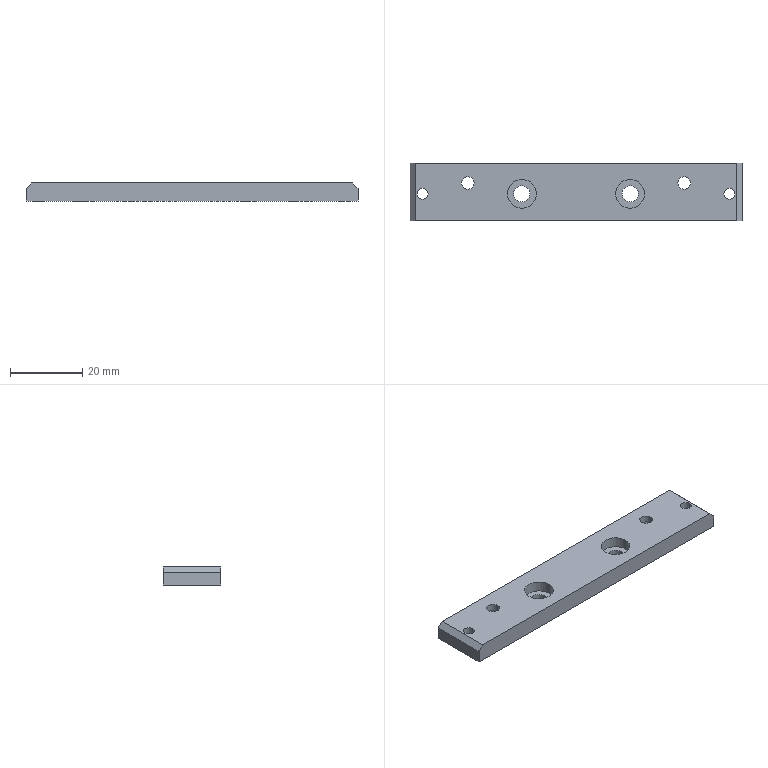Part | NX | 1 solid | 32 faces | box 92 x 16 x 5 mm | volume 6668 mm3 | cylinder 20 | plane 12 | commonest cylinder face diameters 3 x4 3.5 x4 4.5 x4 6.2 x4 8 x4
STEP:
#1=CARTESIAN_POINT('',(-19.,-0.5,-3.));
#2=VERTEX_POINT('',#1);
#3=CARTESIAN_POINT('',(-11.,-0.5,-3.));
#4=VERTEX_POINT('',#3);
#5=CARTESIAN_POINT('',(-15.,-0.5,-3.));
#6=DIRECTION('',(0.,0.,1.));
#7=DIRECTION('',(1.,0.,0.));
#8=AXIS2_PLACEMENT_3D('',#5,#6,#7);
#9=CIRCLE('',#8,4.);
#10=EDGE_CURVE('',#2,#4,#9,.T.);
#11=ORIENTED_EDGE('',*,*,#10,.F.);
#12=CARTESIAN_POINT('',(-19.,-0.5,0.));
#13=VERTEX_POINT('',#12);
#14=CARTESIAN_POINT('',(-19.,-0.5,0.));
#15=DIRECTION('',(0.,0.,1.));
#16=VECTOR('',#15,1000.);
#17=LINE('',#14,#16);
#18=EDGE_CURVE('',#2,#13,#17,.T.);
#19=ORIENTED_EDGE('',*,*,#18,.T.);
#20=CARTESIAN_POINT('',(-11.,-0.5,0.));
#21=VERTEX_POINT('',#20);
#22=CARTESIAN_POINT('',(-15.,-0.5,0.));
#23=DIRECTION('',(0.,0.,1.));
#24=DIRECTION('',(1.,0.,0.));
#25=AXIS2_PLACEMENT_3D('',#22,#23,#24);
#26=CIRCLE('',#25,4.);
#27=EDGE_CURVE('',#13,#21,#26,.T.);
#28=ORIENTED_EDGE('',*,*,#27,.T.);
#29=CARTESIAN_POINT('',(-11.,-0.5,0.));
#30=DIRECTION('',(0.,0.,1.));
#31=VECTOR('',#30,1000.);
#32=LINE('',#29,#31);
#33=EDGE_CURVE('',#4,#21,#32,.T.);
#34=ORIENTED_EDGE('',*,*,#33,.F.);
#35=EDGE_LOOP('',(#11,#19,#28,#34));
#36=FACE_BOUND('',#35,.T.);
#37=CARTESIAN_POINT('',(-15.,-0.5,0.));
#38=DIRECTION('',(0.,0.,1.));
#39=DIRECTION('',(-1.,0.,0.));
#40=AXIS2_PLACEMENT_3D('',#37,#38,#39);
#41=CYLINDRICAL_SURFACE('',#40,4.);
#42=ADVANCED_FACE('',(#36),#41,.F.);
#43=CARTESIAN_POINT('',(-17.25,-0.5,-5.));
#44=VERTEX_POINT('',#43);
#45=CARTESIAN_POINT('',(-12.75,-0.5,-5.));
#46=VERTEX_POINT('',#45);
#47=CARTESIAN_POINT('',(-15.,-0.5,-5.));
#48=DIRECTION('',(0.,0.,1.));
#49=DIRECTION('',(1.,0.,0.));
#50=AXIS2_PLACEMENT_3D('',#47,#48,#49);
#51=CIRCLE('',#50,2.25);
#52=EDGE_CURVE('',#44,#46,#51,.T.);
#53=ORIENTED_EDGE('',*,*,#52,.F.);
#54=CARTESIAN_POINT('',(-17.25,-0.5,-3.));
#55=VERTEX_POINT('',#54);
#56=CARTESIAN_POINT('',(-17.25,-0.5,0.));
#57=DIRECTION('',(0.,0.,1.));
#58=VECTOR('',#57,1000.);
#59=LINE('',#56,#58);
#60=EDGE_CURVE('',#44,#55,#59,.T.);
#61=ORIENTED_EDGE('',*,*,#60,.T.);
#62=CARTESIAN_POINT('',(-12.75,-0.5,-3.));
#63=VERTEX_POINT('',#62);
#64=CARTESIAN_POINT('',(-15.,-0.5,-3.));
#65=DIRECTION('',(0.,0.,1.));
#66=DIRECTION('',(1.,0.,0.));
#67=AXIS2_PLACEMENT_3D('',#64,#65,#66);
#68=CIRCLE('',#67,2.25);
#69=EDGE_CURVE('',#55,#63,#68,.T.);
#70=ORIENTED_EDGE('',*,*,#69,.T.);
#71=CARTESIAN_POINT('',(-12.75,-0.5,0.));
#72=DIRECTION('',(0.,0.,1.));
#73=VECTOR('',#72,1000.);
#74=LINE('',#71,#73);
#75=EDGE_CURVE('',#46,#63,#74,.T.);
#76=ORIENTED_EDGE('',*,*,#75,.F.);
#77=EDGE_LOOP('',(#53,#61,#70,#76));
#78=FACE_BOUND('',#77,.T.);
#79=CARTESIAN_POINT('',(-15.,-0.5,0.));
#80=DIRECTION('',(0.,0.,1.));
#81=DIRECTION('',(-1.,0.,0.));
#82=AXIS2_PLACEMENT_3D('',#79,#80,#81);
#83=CYLINDRICAL_SURFACE('',#82,2.25);
#84=ADVANCED_FACE('',(#78),#83,.F.);
#85=CARTESIAN_POINT('',(11.,-0.5,-3.));
#86=VERTEX_POINT('',#85);
#87=CARTESIAN_POINT('',(19.,-0.5,-3.));
#88=VERTEX_POINT('',#87);
#89=CARTESIAN_POINT('',(15.,-0.5,-3.));
#90=DIRECTION('',(0.,0.,1.));
#91=DIRECTION('',(1.,0.,0.));
#92=AXIS2_PLACEMENT_3D('',#89,#90,#91);
#93=CIRCLE('',#92,4.);
#94=EDGE_CURVE('',#86,#88,#93,.T.);
#95=ORIENTED_EDGE('',*,*,#94,.F.);
#96=CARTESIAN_POINT('',(11.,-0.5,0.));
#97=VERTEX_POINT('',#96);
#98=CARTESIAN_POINT('',(11.,-0.5,0.));
#99=DIRECTION('',(0.,0.,1.));
#100=VECTOR('',#99,1000.);
#101=LINE('',#98,#100);
#102=EDGE_CURVE('',#86,#97,#101,.T.);
#103=ORIENTED_EDGE('',*,*,#102,.T.);
#104=CARTESIAN_POINT('',(19.,-0.5,0.));
#105=VERTEX_POINT('',#104);
#106=CARTESIAN_POINT('',(15.,-0.5,0.));
#107=DIRECTION('',(0.,0.,1.));
#108=DIRECTION('',(1.,0.,0.));
#109=AXIS2_PLACEMENT_3D('',#106,#107,#108);
#110=CIRCLE('',#109,4.);
#111=EDGE_CURVE('',#97,#105,#110,.T.);
#112=ORIENTED_EDGE('',*,*,#111,.T.);
#113=CARTESIAN_POINT('',(19.,-0.5,0.));
#114=DIRECTION('',(0.,0.,1.));
#115=VECTOR('',#114,1000.);
#116=LINE('',#113,#115);
#117=EDGE_CURVE('',#88,#105,#116,.T.);
#118=ORIENTED_EDGE('',*,*,#117,.F.);
#119=EDGE_LOOP('',(#95,#103,#112,#118));
#120=FACE_BOUND('',#119,.T.);
#121=CARTESIAN_POINT('',(15.,-0.5,0.));
#122=DIRECTION('',(0.,0.,1.));
#123=DIRECTION('',(-1.,0.,0.));
#124=AXIS2_PLACEMENT_3D('',#121,#122,#123);
#125=CYLINDRICAL_SURFACE('',#124,4.);
#126=ADVANCED_FACE('',(#120),#125,.F.);
#127=CARTESIAN_POINT('',(12.75,-0.5,-5.));
#128=VERTEX_POINT('',#127);
#129=CARTESIAN_POINT('',(17.25,-0.5,-5.));
#130=VERTEX_POINT('',#129);
#131=CARTESIAN_POINT('',(15.,-0.5,-5.));
#132=DIRECTION('',(0.,0.,1.));
#133=DIRECTION('',(1.,0.,0.));
#134=AXIS2_PLACEMENT_3D('',#131,#132,#133);
#135=CIRCLE('',#134,2.25);
#136=EDGE_CURVE('',#128,#130,#135,.T.);
#137=ORIENTED_EDGE('',*,*,#136,.F.);
#138=CARTESIAN_POINT('',(12.75,-0.5,-3.));
#139=VERTEX_POINT('',#138);
#140=CARTESIAN_POINT('',(12.75,-0.5,0.));
#141=DIRECTION('',(0.,0.,1.));
#142=VECTOR('',#141,1000.);
#143=LINE('',#140,#142);
#144=EDGE_CURVE('',#128,#139,#143,.T.);
#145=ORIENTED_EDGE('',*,*,#144,.T.);
#146=CARTESIAN_POINT('',(17.25,-0.5,-3.));
#147=VERTEX_POINT('',#146);
#148=CARTESIAN_POINT('',(15.,-0.5,-3.));
#149=DIRECTION('',(0.,0.,1.));
#150=DIRECTION('',(1.,0.,0.));
#151=AXIS2_PLACEMENT_3D('',#148,#149,#150);
#152=CIRCLE('',#151,2.25);
#153=EDGE_CURVE('',#139,#147,#152,.T.);
#154=ORIENTED_EDGE('',*,*,#153,.T.);
#155=CARTESIAN_POINT('',(17.25,-0.5,0.));
#156=DIRECTION('',(0.,0.,1.));
#157=VECTOR('',#156,1000.);
#158=LINE('',#155,#157);
#159=EDGE_CURVE('',#130,#147,#158,.T.);
#160=ORIENTED_EDGE('',*,*,#159,.F.);
#161=EDGE_LOOP('',(#137,#145,#154,#160));
#162=FACE_BOUND('',#161,.T.);
#163=CARTESIAN_POINT('',(15.,-0.5,0.));
#164=DIRECTION('',(0.,0.,1.));
#165=DIRECTION('',(-1.,0.,0.));
#166=AXIS2_PLACEMENT_3D('',#163,#164,#165);
#167=CYLINDRICAL_SURFACE('',#166,2.25);
#168=ADVANCED_FACE('',(#162),#167,.F.);
#169=CARTESIAN_POINT('',(-41.,-0.5,0.));
#170=VERTEX_POINT('',#169);
#171=CARTESIAN_POINT('',(-44.,-0.5,0.));
#172=VERTEX_POINT('',#171);
#173=CARTESIAN_POINT('',(-42.5,-0.5,0.));
#174=DIRECTION('',(0.,0.,-1.));
#175=DIRECTION('',(-1.,0.,0.));
#176=AXIS2_PLACEMENT_3D('',#173,#174,#175);
#177=CIRCLE('',#176,1.5);
#178=EDGE_CURVE('',#170,#172,#177,.T.);
#179=ORIENTED_EDGE('',*,*,#178,.F.);
#180=CARTESIAN_POINT('',(-41.,-0.5,-5.));
#181=VERTEX_POINT('',#180);
#182=CARTESIAN_POINT('',(-41.,-0.5,-5.));
#183=DIRECTION('',(0.,0.,-1.));
#184=VECTOR('',#183,1000.);
#185=LINE('',#182,#184);
#186=EDGE_CURVE('',#170,#181,#185,.T.);
#187=ORIENTED_EDGE('',*,*,#186,.T.);
#188=CARTESIAN_POINT('',(-44.,-0.5,-5.));
#189=VERTEX_POINT('',#188);
#190=CARTESIAN_POINT('',(-42.5,-0.5,-5.));
#191=DIRECTION('',(0.,0.,-1.));
#192=DIRECTION('',(-1.,0.,0.));
#193=AXIS2_PLACEMENT_3D('',#190,#191,#192);
#194=CIRCLE('',#193,1.5);
#195=EDGE_CURVE('',#181,#189,#194,.T.);
#196=ORIENTED_EDGE('',*,*,#195,.T.);
#197=CARTESIAN_POINT('',(-44.,-0.5,-5.));
#198=DIRECTION('',(0.,0.,-1.));
#199=VECTOR('',#198,1000.);
#200=LINE('',#197,#199);
#201=EDGE_CURVE('',#172,#189,#200,.T.);
#202=ORIENTED_EDGE('',*,*,#201,.F.);
#203=EDGE_LOOP('',(#179,#187,#196,#202));
#204=FACE_BOUND('',#203,.T.);
#205=CARTESIAN_POINT('',(-42.5,-0.5,-5.));
#206=DIRECTION('',(0.,0.,-1.));
#207=DIRECTION('',(1.,0.,0.));
#208=AXIS2_PLACEMENT_3D('',#205,#206,#207);
#209=CYLINDRICAL_SURFACE('',#208,1.5);
#210=ADVANCED_FACE('',(#204),#209,.F.);
#211=CARTESIAN_POINT('',(44.,-0.5,0.));
#212=VERTEX_POINT('',#211);
#213=CARTESIAN_POINT('',(41.,-0.5,0.));
#214=VERTEX_POINT('',#213);
#215=CARTESIAN_POINT('',(42.5,-0.5,0.));
#216=DIRECTION('',(0.,0.,-1.));
#217=DIRECTION('',(-1.,0.,0.));
#218=AXIS2_PLACEMENT_3D('',#215,#216,#217);
#219=CIRCLE('',#218,1.5);
#220=EDGE_CURVE('',#212,#214,#219,.T.);
#221=ORIENTED_EDGE('',*,*,#220,.F.);
#222=CARTESIAN_POINT('',(44.,-0.5,-5.));
#223=VERTEX_POINT('',#222);
#224=CARTESIAN_POINT('',(44.,-0.5,-5.));
#225=DIRECTION('',(0.,0.,-1.));
#226=VECTOR('',#225,1000.);
#227=LINE('',#224,#226);
#228=EDGE_CURVE('',#212,#223,#227,.T.);
#229=ORIENTED_EDGE('',*,*,#228,.T.);
#230=CARTESIAN_POINT('',(41.,-0.5,-5.));
#231=VERTEX_POINT('',#230);
#232=CARTESIAN_POINT('',(42.5,-0.5,-5.));
#233=DIRECTION('',(0.,0.,-1.));
#234=DIRECTION('',(-1.,0.,0.));
#235=AXIS2_PLACEMENT_3D('',#232,#233,#234);
#236=CIRCLE('',#235,1.5);
#237=EDGE_CURVE('',#223,#231,#236,.T.);
#238=ORIENTED_EDGE('',*,*,#237,.T.);
#239=CARTESIAN_POINT('',(41.,-0.5,-5.));
#240=DIRECTION('',(0.,0.,-1.));
#241=VECTOR('',#240,1000.);
#242=LINE('',#239,#241);
#243=EDGE_CURVE('',#214,#231,#242,.T.);
#244=ORIENTED_EDGE('',*,*,#243,.F.);
#245=EDGE_LOOP('',(#221,#229,#238,#244));
#246=FACE_BOUND('',#245,.T.);
#247=CARTESIAN_POINT('',(42.5,-0.5,-5.));
#248=DIRECTION('',(0.,0.,-1.));
#249=DIRECTION('',(1.,0.,0.));
#250=AXIS2_PLACEMENT_3D('',#247,#248,#249);
#251=CYLINDRICAL_SURFACE('',#250,1.5);
#252=ADVANCED_FACE('',(#246),#251,.F.);
#253=CARTESIAN_POINT('',(-31.75,2.5,0.));
#254=VERTEX_POINT('',#253);
#255=CARTESIAN_POINT('',(-28.25,2.5,0.));
#256=VERTEX_POINT('',#255);
#257=CARTESIAN_POINT('',(-30.,2.5,0.));
#258=DIRECTION('',(0.,0.,1.));
#259=DIRECTION('',(1.,0.,0.));
#260=AXIS2_PLACEMENT_3D('',#257,#258,#259);
#261=CIRCLE('',#260,1.75);
#262=EDGE_CURVE('',#254,#256,#261,.T.);
#263=ORIENTED_EDGE('',*,*,#262,.T.);
#264=CARTESIAN_POINT('',(-28.25,2.5,-2.));
#265=VERTEX_POINT('',#264);
#266=CARTESIAN_POINT('',(-28.25,2.5,-2.));
#267=DIRECTION('',(0.,0.,-1.));
#268=VECTOR('',#267,1000.);
#269=LINE('',#266,#268);
#270=EDGE_CURVE('',#256,#265,#269,.T.);
#271=ORIENTED_EDGE('',*,*,#270,.T.);
#272=CARTESIAN_POINT('',(-31.75,2.5,-2.));
#273=VERTEX_POINT('',#272);
#274=CARTESIAN_POINT('',(-30.,2.5,-2.));
#275=DIRECTION('',(0.,0.,-1.));
#276=DIRECTION('',(-1.,0.,0.));
#277=AXIS2_PLACEMENT_3D('',#274,#275,#276);
#278=CIRCLE('',#277,1.75);
#279=EDGE_CURVE('',#265,#273,#278,.T.);
#280=ORIENTED_EDGE('',*,*,#279,.T.);
#281=CARTESIAN_POINT('',(-31.75,2.5,-2.));
#282=DIRECTION('',(0.,0.,-1.));
#283=VECTOR('',#282,1000.);
#284=LINE('',#281,#283);
#285=EDGE_CURVE('',#254,#273,#284,.T.);
#286=ORIENTED_EDGE('',*,*,#285,.F.);
#287=EDGE_LOOP('',(#263,#271,#280,#286));
#288=FACE_BOUND('',#287,.T.);
#289=CARTESIAN_POINT('',(-30.,2.5,-2.));
#290=DIRECTION('',(0.,0.,-1.));
#291=DIRECTION('',(1.,0.,0.));
#292=AXIS2_PLACEMENT_3D('',#289,#290,#291);
#293=CYLINDRICAL_SURFACE('',#292,1.75);
#294=ADVANCED_FACE('',(#288),#293,.F.);
#295=CARTESIAN_POINT('',(28.25,2.5,0.));
#296=VERTEX_POINT('',#295);
#297=CARTESIAN_POINT('',(31.75,2.5,0.));
#298=VERTEX_POINT('',#297);
#299=CARTESIAN_POINT('',(30.,2.5,0.));
#300=DIRECTION('',(0.,0.,1.));
#301=DIRECTION('',(1.,0.,0.));
#302=AXIS2_PLACEMENT_3D('',#299,#300,#301);
#303=CIRCLE('',#302,1.75);
#304=EDGE_CURVE('',#296,#298,#303,.T.);
#305=ORIENTED_EDGE('',*,*,#304,.T.);
#306=CARTESIAN_POINT('',(31.75,2.5,-2.));
#307=VERTEX_POINT('',#306);
#308=CARTESIAN_POINT('',(31.75,2.5,-2.));
#309=DIRECTION('',(0.,0.,-1.));
#310=VECTOR('',#309,1000.);
#311=LINE('',#308,#310);
#312=EDGE_CURVE('',#298,#307,#311,.T.);
#313=ORIENTED_EDGE('',*,*,#312,.T.);
#314=CARTESIAN_POINT('',(28.25,2.5,-2.));
#315=VERTEX_POINT('',#314);
#316=CARTESIAN_POINT('',(30.,2.5,-2.));
#317=DIRECTION('',(0.,0.,-1.));
#318=DIRECTION('',(-1.,0.,0.));
#319=AXIS2_PLACEMENT_3D('',#316,#317,#318);
#320=CIRCLE('',#319,1.75);
#321=EDGE_CURVE('',#307,#315,#320,.T.);
#322=ORIENTED_EDGE('',*,*,#321,.T.);
#323=CARTESIAN_POINT('',(28.25,2.5,-2.));
#324=DIRECTION('',(0.,0.,-1.));
#325=VECTOR('',#324,1000.);
#326=LINE('',#323,#325);
#327=EDGE_CURVE('',#296,#315,#326,.T.);
#328=ORIENTED_EDGE('',*,*,#327,.F.);
#329=EDGE_LOOP('',(#305,#313,#322,#328));
#330=FACE_BOUND('',#329,.T.);
#331=CARTESIAN_POINT('',(30.,2.5,-2.));
#332=DIRECTION('',(0.,0.,-1.));
#333=DIRECTION('',(1.,0.,0.));
#334=AXIS2_PLACEMENT_3D('',#331,#332,#333);
#335=CYLINDRICAL_SURFACE('',#334,1.75);
#336=ADVANCED_FACE('',(#330),#335,.F.);
#337=CARTESIAN_POINT('',(26.9,2.5,-2.));
#338=VERTEX_POINT('',#337);
#339=CARTESIAN_POINT('',(33.1,2.5,-2.));
#340=VERTEX_POINT('',#339);
#341=CARTESIAN_POINT('',(30.,2.5,-2.));
#342=DIRECTION('',(0.,0.,1.));
#343=DIRECTION('',(1.,0.,0.));
#344=AXIS2_PLACEMENT_3D('',#341,#342,#343);
#345=CIRCLE('',#344,3.1);
#346=EDGE_CURVE('',#338,#340,#345,.T.);
#347=ORIENTED_EDGE('',*,*,#346,.T.);
#348=CARTESIAN_POINT('',(33.1,2.5,-5.));
#349=VERTEX_POINT('',#348);
#350=CARTESIAN_POINT('',(33.1,2.5,-2.));
#351=DIRECTION('',(0.,0.,-1.));
#352=VECTOR('',#351,1000.);
#353=LINE('',#350,#352);
#354=EDGE_CURVE('',#340,#349,#353,.T.);
#355=ORIENTED_EDGE('',*,*,#354,.T.);
#356=CARTESIAN_POINT('',(26.9,2.5,-5.));
#357=VERTEX_POINT('',#356);
#358=CARTESIAN_POINT('',(30.,2.5,-5.));
#359=DIRECTION('',(0.,0.,1.));
#360=DIRECTION('',(1.,0.,0.));
#361=AXIS2_PLACEMENT_3D('',#358,#359,#360);
#362=CIRCLE('',#361,3.1);
#363=EDGE_CURVE('',#357,#349,#362,.T.);
#364=ORIENTED_EDGE('',*,*,#363,.F.);
#365=CARTESIAN_POINT('',(26.9,2.5,-2.));
#366=DIRECTION('',(0.,0.,-1.));
#367=VECTOR('',#366,1000.);
#368=LINE('',#365,#367);
#369=EDGE_CURVE('',#338,#357,#368,.T.);
#370=ORIENTED_EDGE('',*,*,#369,.F.);
#371=EDGE_LOOP('',(#347,#355,#364,#370));
#372=FACE_BOUND('',#371,.T.);
#373=CARTESIAN_POINT('',(30.,2.5,-2.));
#374=DIRECTION('',(0.,0.,-1.));
#375=DIRECTION('',(1.,0.,0.));
#376=AXIS2_PLACEMENT_3D('',#373,#374,#375);
#377=CYLINDRICAL_SURFACE('',#376,3.1);
#378=ADVANCED_FACE('',(#372),#377,.F.);
#379=CARTESIAN_POINT('',(-33.1,2.5,-2.));
#380=VERTEX_POINT('',#379);
#381=CARTESIAN_POINT('',(-26.9,2.5,-2.));
#382=VERTEX_POINT('',#381);
#383=CARTESIAN_POINT('',(-30.,2.5,-2.));
#384=DIRECTION('',(0.,0.,1.));
#385=DIRECTION('',(1.,0.,0.));
#386=AXIS2_PLACEMENT_3D('',#383,#384,#385);
#387=CIRCLE('',#386,3.1);
#388=EDGE_CURVE('',#380,#382,#387,.T.);
#389=ORIENTED_EDGE('',*,*,#388,.T.);
#390=CARTESIAN_POINT('',(-26.9,2.5,-5.));
#391=VERTEX_POINT('',#390);
#392=CARTESIAN_POINT('',(-26.9,2.5,-2.));
#393=DIRECTION('',(0.,0.,-1.));
#394=VECTOR('',#393,1000.);
#395=LINE('',#392,#394);
#396=EDGE_CURVE('',#382,#391,#395,.T.);
#397=ORIENTED_EDGE('',*,*,#396,.T.);
#398=CARTESIAN_POINT('',(-33.1,2.5,-5.));
#399=VERTEX_POINT('',#398);
#400=CARTESIAN_POINT('',(-30.,2.5,-5.));
#401=DIRECTION('',(0.,0.,1.));
#402=DIRECTION('',(1.,0.,0.));
#403=AXIS2_PLACEMENT_3D('',#400,#401,#402);
#404=CIRCLE('',#403,3.1);
#405=EDGE_CURVE('',#399,#391,#404,.T.);
#406=ORIENTED_EDGE('',*,*,#405,.F.);
#407=CARTESIAN_POINT('',(-33.1,2.5,-2.));
#408=DIRECTION('',(0.,0.,-1.));
#409=VECTOR('',#408,1000.);
#410=LINE('',#407,#409);
#411=EDGE_CURVE('',#380,#399,#410,.T.);
#412=ORIENTED_EDGE('',*,*,#411,.F.);
#413=EDGE_LOOP('',(#389,#397,#406,#412));
#414=FACE_BOUND('',#413,.T.);
#415=CARTESIAN_POINT('',(-30.,2.5,-2.));
#416=DIRECTION('',(0.,0.,-1.));
#417=DIRECTION('',(1.,0.,0.));
#418=AXIS2_PLACEMENT_3D('',#415,#416,#417);
#419=CYLINDRICAL_SURFACE('',#418,3.1);
#420=ADVANCED_FACE('',(#414),#419,.F.);
#421=ORIENTED_EDGE('',*,*,#388,.F.);
#422=CARTESIAN_POINT('',(-30.,2.5,-2.));
#423=DIRECTION('',(0.,0.,1.));
#424=DIRECTION('',(1.,0.,0.));
#425=AXIS2_PLACEMENT_3D('',#422,#423,#424);
#426=CIRCLE('',#425,3.1);
#427=EDGE_CURVE('',#382,#380,#426,.T.);
#428=ORIENTED_EDGE('',*,*,#427,.F.);
#429=EDGE_LOOP('',(#421,#428));
#430=FACE_BOUND('',#429,.T.);
#431=CARTESIAN_POINT('',(-30.,2.5,-2.));
#432=DIRECTION('',(0.,0.,-1.));
#433=DIRECTION('',(-1.,0.,0.));
#434=AXIS2_PLACEMENT_3D('',#431,#432,#433);
#435=CIRCLE('',#434,1.75);
#436=EDGE_CURVE('',#273,#265,#435,.T.);
#437=ORIENTED_EDGE('',*,*,#436,.F.);
#438=ORIENTED_EDGE('',*,*,#279,.F.);
#439=EDGE_LOOP('',(#437,#438));
#440=FACE_BOUND('',#439,.T.);
#441=CARTESIAN_POINT('',(-30.,2.5,-2.));
#442=DIRECTION('',(0.,0.,1.));
#443=DIRECTION('',(-1.,0.,0.));
#444=AXIS2_PLACEMENT_3D('',#441,#442,#443);
#445=PLANE('',#444);
#446=ADVANCED_FACE('',(#430,#440),#445,.F.);
#447=CARTESIAN_POINT('',(46.,8.,-1.5));
#448=VERTEX_POINT('',#447);
#449=CARTESIAN_POINT('',(46.,8.,-5.));
#450=VERTEX_POINT('',#449);
#451=CARTESIAN_POINT('',(46.,8.,0.));
#452=DIRECTION('',(0.,0.,-1.));
#453=VECTOR('',#452,1000.);
#454=LINE('',#451,#453);
#455=EDGE_CURVE('',#448,#450,#454,.T.);
#456=ORIENTED_EDGE('',*,*,#455,.F.);
#457=CARTESIAN_POINT('',(46.,-8.,-1.5));
#458=VERTEX_POINT('',#457);
#459=CARTESIAN_POINT('',(46.,-8.,-1.5));
#460=DIRECTION('',(0.,-1.,0.));
#461=VECTOR('',#460,1000.);
#462=LINE('',#459,#461);
#463=EDGE_CURVE('',#448,#458,#462,.T.);
#464=ORIENTED_EDGE('',*,*,#463,.T.);
#465=CARTESIAN_POINT('',(46.,-8.,-5.));
#466=VERTEX_POINT('',#465);
#467=CARTESIAN_POINT('',(46.,-8.,0.));
#468=DIRECTION('',(0.,0.,-1.));
#469=VECTOR('',#468,1000.);
#470=LINE('',#467,#469);
#471=EDGE_CURVE('',#458,#466,#470,.T.);
#472=ORIENTED_EDGE('',*,*,#471,.T.);
#473=CARTESIAN_POINT('',(46.,8.,-5.));
#474=DIRECTION('',(0.,1.,0.));
#475=VECTOR('',#474,1000.);
#476=LINE('',#473,#475);
#477=EDGE_CURVE('',#466,#450,#476,.T.);
#478=ORIENTED_EDGE('',*,*,#477,.T.);
#479=EDGE_LOOP('',(#456,#464,#472,#478));
#480=FACE_BOUND('',#479,.T.);
#481=CARTESIAN_POINT('',(46.,8.,0.));
#482=DIRECTION('',(-1.,0.,0.));
#483=DIRECTION('',(0.,0.,-1.));
#484=AXIS2_PLACEMENT_3D('',#481,#482,#483);
#485=PLANE('',#484);
#486=ADVANCED_FACE('',(#480),#485,.F.);
#487=CARTESIAN_POINT('',(-46.,8.,-1.5));
#488=VERTEX_POINT('',#487);
#489=CARTESIAN_POINT('',(-46.,8.,-5.));
#490=VERTEX_POINT('',#489);
#491=CARTESIAN_POINT('',(-46.,8.,0.));
#492=DIRECTION('',(0.,0.,-1.));
#493=VECTOR('',#492,1000.);
#494=LINE('',#491,#493);
#495=EDGE_CURVE('',#488,#490,#494,.T.);
#496=ORIENTED_EDGE('',*,*,#495,.F.);
#497=CARTESIAN_POINT('',(-44.5,8.,0.));
#498=VERTEX_POINT('',#497);
#499=CARTESIAN_POINT('',(-44.5,8.,0.));
#500=DIRECTION('',(0.7071,0.,0.7071));
#501=VECTOR('',#500,1000.);
#502=LINE('',#499,#501);
#503=EDGE_CURVE('',#488,#498,#502,.T.);
#504=ORIENTED_EDGE('',*,*,#503,.T.);
#505=CARTESIAN_POINT('',(44.5,8.,0.));
#506=VERTEX_POINT('',#505);
#507=CARTESIAN_POINT('',(-46.,8.,0.));
#508=DIRECTION('',(-1.,0.,0.));
#509=VECTOR('',#508,1000.);
#510=LINE('',#507,#509);
#511=EDGE_CURVE('',#506,#498,#510,.T.);
#512=ORIENTED_EDGE('',*,*,#511,.F.);
#513=CARTESIAN_POINT('',(44.5,8.,0.));
#514=DIRECTION('',(0.7071,0.,-0.7071));
#515=VECTOR('',#514,1000.);
#516=LINE('',#513,#515);
#517=EDGE_CURVE('',#506,#448,#516,.T.);
#518=ORIENTED_EDGE('',*,*,#517,.T.);
#519=ORIENTED_EDGE('',*,*,#455,.T.);
#520=CARTESIAN_POINT('',(-46.,8.,-5.));
#521=DIRECTION('',(-1.,0.,0.));
#522=VECTOR('',#521,1000.);
#523=LINE('',#520,#522);
#524=EDGE_CURVE('',#450,#490,#523,.T.);
#525=ORIENTED_EDGE('',*,*,#524,.T.);
#526=EDGE_LOOP('',(#496,#504,#512,#518,#519,#525));
#527=FACE_BOUND('',#526,.T.);
#528=CARTESIAN_POINT('',(-46.,8.,0.));
#529=DIRECTION('',(0.,-1.,0.));
#530=DIRECTION('',(0.,0.,1.));
#531=AXIS2_PLACEMENT_3D('',#528,#529,#530);
#532=PLANE('',#531);
#533=ADVANCED_FACE('',(#527),#532,.F.);
#534=CARTESIAN_POINT('',(-46.,-8.,-1.5));
#535=VERTEX_POINT('',#534);
#536=CARTESIAN_POINT('',(-46.,-8.,-5.));
#537=VERTEX_POINT('',#536);
#538=CARTESIAN_POINT('',(-46.,-8.,0.));
#539=DIRECTION('',(0.,0.,-1.));
#540=VECTOR('',#539,1000.);
#541=LINE('',#538,#540);
#542=EDGE_CURVE('',#535,#537,#541,.T.);
#543=ORIENTED_EDGE('',*,*,#542,.F.);
#544=CARTESIAN_POINT('',(-46.,8.,-1.5));
#545=DIRECTION('',(0.,1.,0.));
#546=VECTOR('',#545,1000.);
#547=LINE('',#544,#546);
#548=EDGE_CURVE('',#535,#488,#547,.T.);
#549=ORIENTED_EDGE('',*,*,#548,.T.);
#550=ORIENTED_EDGE('',*,*,#495,.T.);
#551=CARTESIAN_POINT('',(-46.,8.,-5.));
#552=DIRECTION('',(0.,-1.,0.));
#553=VECTOR('',#552,1000.);
#554=LINE('',#551,#553);
#555=EDGE_CURVE('',#490,#537,#554,.T.);
#556=ORIENTED_EDGE('',*,*,#555,.T.);
#557=EDGE_LOOP('',(#543,#549,#550,#556));
#558=FACE_BOUND('',#557,.T.);
#559=CARTESIAN_POINT('',(-46.,8.,0.));
#560=DIRECTION('',(1.,0.,0.));
#561=DIRECTION('',(0.,0.,1.));
#562=AXIS2_PLACEMENT_3D('',#559,#560,#561);
#563=PLANE('',#562);
#564=ADVANCED_FACE('',(#558),#563,.F.);
#565=CARTESIAN_POINT('',(-44.5,-8.,0.));
#566=VERTEX_POINT('',#565);
#567=CARTESIAN_POINT('',(44.5,-8.,0.));
#568=VERTEX_POINT('',#567);
#569=CARTESIAN_POINT('',(-46.,-8.,0.));
#570=DIRECTION('',(1.,0.,0.));
#571=VECTOR('',#570,1000.);
#572=LINE('',#569,#571);
#573=EDGE_CURVE('',#566,#568,#572,.T.);
#574=ORIENTED_EDGE('',*,*,#573,.F.);
#575=CARTESIAN_POINT('',(-44.5,-8.,0.));
#576=DIRECTION('',(-0.7071,0.,-0.7071));
#577=VECTOR('',#576,1000.);
#578=LINE('',#575,#577);
#579=EDGE_CURVE('',#566,#535,#578,.T.);
#580=ORIENTED_EDGE('',*,*,#579,.T.);
#581=ORIENTED_EDGE('',*,*,#542,.T.);
#582=CARTESIAN_POINT('',(-46.,-8.,-5.));
#583=DIRECTION('',(1.,0.,0.));
#584=VECTOR('',#583,1000.);
#585=LINE('',#582,#584);
#586=EDGE_CURVE('',#537,#466,#585,.T.);
#587=ORIENTED_EDGE('',*,*,#586,.T.);
#588=ORIENTED_EDGE('',*,*,#471,.F.);
#589=CARTESIAN_POINT('',(44.5,-8.,0.));
#590=DIRECTION('',(-0.7071,0.,0.7071));
#591=VECTOR('',#590,1000.);
#592=LINE('',#589,#591);
#593=EDGE_CURVE('',#458,#568,#592,.T.);
#594=ORIENTED_EDGE('',*,*,#593,.T.);
#595=EDGE_LOOP('',(#574,#580,#581,#587,#588,#594));
#596=FACE_BOUND('',#595,.T.);
#597=CARTESIAN_POINT('',(-46.,-8.,0.));
#598=DIRECTION('',(0.,1.,0.));
#599=DIRECTION('',(0.,0.,-1.));
#600=AXIS2_PLACEMENT_3D('',#597,#598,#599);
#601=PLANE('',#600);
#602=ADVANCED_FACE('',(#596),#601,.F.);
#603=CARTESIAN_POINT('',(-15.,-0.5,0.));
#604=DIRECTION('',(0.,0.,1.));
#605=DIRECTION('',(1.,0.,0.));
#606=AXIS2_PLACEMENT_3D('',#603,#604,#605);
#607=CIRCLE('',#606,4.);
#608=EDGE_CURVE('',#21,#13,#607,.T.);
#609=ORIENTED_EDGE('',*,*,#608,.F.);
#610=ORIENTED_EDGE('',*,*,#27,.F.);
#611=EDGE_LOOP('',(#609,#610));
#612=FACE_BOUND('',#611,.T.);
#613=CARTESIAN_POINT('',(15.,-0.5,0.));
#614=DIRECTION('',(0.,0.,1.));
#615=DIRECTION('',(1.,0.,0.));
#616=AXIS2_PLACEMENT_3D('',#613,#614,#615);
#617=CIRCLE('',#616,4.);
#618=EDGE_CURVE('',#105,#97,#617,.T.);
#619=ORIENTED_EDGE('',*,*,#618,.F.);
#620=ORIENTED_EDGE('',*,*,#111,.F.);
#621=EDGE_LOOP('',(#619,#620));
#622=FACE_BOUND('',#621,.T.);
#623=CARTESIAN_POINT('',(-42.5,-0.5,0.));
#624=DIRECTION('',(0.,0.,-1.));
#625=DIRECTION('',(-1.,0.,0.));
#626=AXIS2_PLACEMENT_3D('',#623,#624,#625);
#627=CIRCLE('',#626,1.5);
#628=EDGE_CURVE('',#172,#170,#627,.T.);
#629=ORIENTED_EDGE('',*,*,#628,.T.);
#630=ORIENTED_EDGE('',*,*,#178,.T.);
#631=EDGE_LOOP('',(#629,#630));
#632=FACE_BOUND('',#631,.T.);
#633=CARTESIAN_POINT('',(42.5,-0.5,0.));
#634=DIRECTION('',(0.,0.,-1.));
#635=DIRECTION('',(-1.,0.,0.));
#636=AXIS2_PLACEMENT_3D('',#633,#634,#635);
#637=CIRCLE('',#636,1.5);
#638=EDGE_CURVE('',#214,#212,#637,.T.);
#639=ORIENTED_EDGE('',*,*,#638,.T.);
#640=ORIENTED_EDGE('',*,*,#220,.T.);
#641=EDGE_LOOP('',(#639,#640));
#642=FACE_BOUND('',#641,.T.);
#643=ORIENTED_EDGE('',*,*,#262,.F.);
#644=CARTESIAN_POINT('',(-30.,2.5,0.));
#645=DIRECTION('',(0.,0.,1.));
#646=DIRECTION('',(1.,0.,0.));
#647=AXIS2_PLACEMENT_3D('',#644,#645,#646);
#648=CIRCLE('',#647,1.75);
#649=EDGE_CURVE('',#256,#254,#648,.T.);
#650=ORIENTED_EDGE('',*,*,#649,.F.);
#651=EDGE_LOOP('',(#643,#650));
#652=FACE_BOUND('',#651,.T.);
#653=ORIENTED_EDGE('',*,*,#304,.F.);
#654=CARTESIAN_POINT('',(30.,2.5,0.));
#655=DIRECTION('',(0.,0.,1.));
#656=DIRECTION('',(1.,0.,0.));
#657=AXIS2_PLACEMENT_3D('',#654,#655,#656);
#658=CIRCLE('',#657,1.75);
#659=EDGE_CURVE('',#298,#296,#658,.T.);
#660=ORIENTED_EDGE('',*,*,#659,.F.);
#661=EDGE_LOOP('',(#653,#660));
#662=FACE_BOUND('',#661,.T.);
#663=ORIENTED_EDGE('',*,*,#511,.T.);
#664=CARTESIAN_POINT('',(-44.5,-8.,0.));
#665=DIRECTION('',(0.,-1.,0.));
#666=VECTOR('',#665,1000.);
#667=LINE('',#664,#666);
#668=EDGE_CURVE('',#498,#566,#667,.T.);
#669=ORIENTED_EDGE('',*,*,#668,.T.);
#670=ORIENTED_EDGE('',*,*,#573,.T.);
#671=CARTESIAN_POINT('',(44.5,8.,0.));
#672=DIRECTION('',(0.,1.,0.));
#673=VECTOR('',#672,1000.);
#674=LINE('',#671,#673);
#675=EDGE_CURVE('',#568,#506,#674,.T.);
#676=ORIENTED_EDGE('',*,*,#675,.T.);
#677=EDGE_LOOP('',(#663,#669,#670,#676));
#678=FACE_BOUND('',#677,.T.);
#679=CARTESIAN_POINT('',(0.,0.,0.));
#680=DIRECTION('',(0.,0.,1.));
#681=DIRECTION('',(-1.,0.,0.));
#682=AXIS2_PLACEMENT_3D('',#679,#680,#681);
#683=PLANE('',#682);
#684=ADVANCED_FACE('',(#612,#622,#632,#642,#652,#662,#678),#683,.T.);
#685=CARTESIAN_POINT('',(-15.,-0.5,-5.));
#686=DIRECTION('',(0.,0.,1.));
#687=DIRECTION('',(1.,0.,0.));
#688=AXIS2_PLACEMENT_3D('',#685,#686,#687);
#689=CIRCLE('',#688,2.25);
#690=EDGE_CURVE('',#46,#44,#689,.T.);
#691=ORIENTED_EDGE('',*,*,#690,.T.);
#692=ORIENTED_EDGE('',*,*,#52,.T.);
#693=EDGE_LOOP('',(#691,#692));
#694=FACE_BOUND('',#693,.T.);
#695=CARTESIAN_POINT('',(15.,-0.5,-5.));
#696=DIRECTION('',(0.,0.,1.));
#697=DIRECTION('',(1.,0.,0.));
#698=AXIS2_PLACEMENT_3D('',#695,#696,#697);
#699=CIRCLE('',#698,2.25);
#700=EDGE_CURVE('',#130,#128,#699,.T.);
#701=ORIENTED_EDGE('',*,*,#700,.T.);
#702=ORIENTED_EDGE('',*,*,#136,.T.);
#703=EDGE_LOOP('',(#701,#702));
#704=FACE_BOUND('',#703,.T.);
#705=CARTESIAN_POINT('',(-42.5,-0.5,-5.));
#706=DIRECTION('',(0.,0.,-1.));
#707=DIRECTION('',(-1.,0.,0.));
#708=AXIS2_PLACEMENT_3D('',#705,#706,#707);
#709=CIRCLE('',#708,1.5);
#710=EDGE_CURVE('',#189,#181,#709,.T.);
#711=ORIENTED_EDGE('',*,*,#710,.F.);
#712=ORIENTED_EDGE('',*,*,#195,.F.);
#713=EDGE_LOOP('',(#711,#712));
#714=FACE_BOUND('',#713,.T.);
#715=CARTESIAN_POINT('',(42.5,-0.5,-5.));
#716=DIRECTION('',(0.,0.,-1.));
#717=DIRECTION('',(-1.,0.,0.));
#718=AXIS2_PLACEMENT_3D('',#715,#716,#717);
#719=CIRCLE('',#718,1.5);
#720=EDGE_CURVE('',#231,#223,#719,.T.);
#721=ORIENTED_EDGE('',*,*,#720,.F.);
#722=ORIENTED_EDGE('',*,*,#237,.F.);
#723=EDGE_LOOP('',(#721,#722));
#724=FACE_BOUND('',#723,.T.);
#725=ORIENTED_EDGE('',*,*,#363,.T.);
#726=CARTESIAN_POINT('',(30.,2.5,-5.));
#727=DIRECTION('',(0.,0.,1.));
#728=DIRECTION('',(1.,0.,0.));
#729=AXIS2_PLACEMENT_3D('',#726,#727,#728);
#730=CIRCLE('',#729,3.1);
#731=EDGE_CURVE('',#349,#357,#730,.T.);
#732=ORIENTED_EDGE('',*,*,#731,.T.);
#733=EDGE_LOOP('',(#725,#732));
#734=FACE_BOUND('',#733,.T.);
#735=ORIENTED_EDGE('',*,*,#405,.T.);
#736=CARTESIAN_POINT('',(-30.,2.5,-5.));
#737=DIRECTION('',(0.,0.,1.));
#738=DIRECTION('',(1.,0.,0.));
#739=AXIS2_PLACEMENT_3D('',#736,#737,#738);
#740=CIRCLE('',#739,3.1);
#741=EDGE_CURVE('',#391,#399,#740,.T.);
#742=ORIENTED_EDGE('',*,*,#741,.T.);
#743=EDGE_LOOP('',(#735,#742));
#744=FACE_BOUND('',#743,.T.);
#745=ORIENTED_EDGE('',*,*,#477,.F.);
#746=ORIENTED_EDGE('',*,*,#586,.F.);
#747=ORIENTED_EDGE('',*,*,#555,.F.);
#748=ORIENTED_EDGE('',*,*,#524,.F.);
#749=EDGE_LOOP('',(#745,#746,#747,#748));
#750=FACE_BOUND('',#749,.T.);
#751=CARTESIAN_POINT('',(0.,0.,-5.));
#752=DIRECTION('',(0.,0.,1.));
#753=DIRECTION('',(-1.,0.,0.));
#754=AXIS2_PLACEMENT_3D('',#751,#752,#753);
#755=PLANE('',#754);
#756=ADVANCED_FACE('',(#694,#704,#714,#724,#734,#744,#750),#755,.F.);
#757=ORIENTED_EDGE('',*,*,#396,.F.);
#758=ORIENTED_EDGE('',*,*,#427,.T.);
#759=ORIENTED_EDGE('',*,*,#411,.T.);
#760=ORIENTED_EDGE('',*,*,#741,.F.);
#761=EDGE_LOOP('',(#757,#758,#759,#760));
#762=FACE_BOUND('',#761,.T.);
#763=CARTESIAN_POINT('',(-30.,2.5,-2.));
#764=DIRECTION('',(0.,0.,-1.));
#765=DIRECTION('',(1.,0.,0.));
#766=AXIS2_PLACEMENT_3D('',#763,#764,#765);
#767=CYLINDRICAL_SURFACE('',#766,3.1);
#768=ADVANCED_FACE('',(#762),#767,.F.);
#769=ORIENTED_EDGE('',*,*,#354,.F.);
#770=CARTESIAN_POINT('',(30.,2.5,-2.));
#771=DIRECTION('',(0.,0.,1.));
#772=DIRECTION('',(1.,0.,0.));
#773=AXIS2_PLACEMENT_3D('',#770,#771,#772);
#774=CIRCLE('',#773,3.1);
#775=EDGE_CURVE('',#340,#338,#774,.T.);
#776=ORIENTED_EDGE('',*,*,#775,.T.);
#777=ORIENTED_EDGE('',*,*,#369,.T.);
#778=ORIENTED_EDGE('',*,*,#731,.F.);
#779=EDGE_LOOP('',(#769,#776,#777,#778));
#780=FACE_BOUND('',#779,.T.);
#781=CARTESIAN_POINT('',(30.,2.5,-2.));
#782=DIRECTION('',(0.,0.,-1.));
#783=DIRECTION('',(1.,0.,0.));
#784=AXIS2_PLACEMENT_3D('',#781,#782,#783);
#785=CYLINDRICAL_SURFACE('',#784,3.1);
#786=ADVANCED_FACE('',(#780),#785,.F.);
#787=CARTESIAN_POINT('',(30.,2.5,-2.));
#788=DIRECTION('',(0.,0.,-1.));
#789=DIRECTION('',(-1.,0.,0.));
#790=AXIS2_PLACEMENT_3D('',#787,#788,#789);
#791=CIRCLE('',#790,1.75);
#792=EDGE_CURVE('',#315,#307,#791,.T.);
#793=ORIENTED_EDGE('',*,*,#792,.F.);
#794=ORIENTED_EDGE('',*,*,#321,.F.);
#795=EDGE_LOOP('',(#793,#794));
#796=FACE_BOUND('',#795,.T.);
#797=ORIENTED_EDGE('',*,*,#346,.F.);
#798=ORIENTED_EDGE('',*,*,#775,.F.);
#799=EDGE_LOOP('',(#797,#798));
#800=FACE_BOUND('',#799,.T.);
#801=CARTESIAN_POINT('',(30.,2.5,-2.));
#802=DIRECTION('',(0.,0.,1.));
#803=DIRECTION('',(-1.,0.,0.));
#804=AXIS2_PLACEMENT_3D('',#801,#802,#803);
#805=PLANE('',#804);
#806=ADVANCED_FACE('',(#796,#800),#805,.F.);
#807=ORIENTED_EDGE('',*,*,#312,.F.);
#808=ORIENTED_EDGE('',*,*,#659,.T.);
#809=ORIENTED_EDGE('',*,*,#327,.T.);
#810=ORIENTED_EDGE('',*,*,#792,.T.);
#811=EDGE_LOOP('',(#807,#808,#809,#810));
#812=FACE_BOUND('',#811,.T.);
#813=CARTESIAN_POINT('',(30.,2.5,-2.));
#814=DIRECTION('',(0.,0.,-1.));
#815=DIRECTION('',(1.,0.,0.));
#816=AXIS2_PLACEMENT_3D('',#813,#814,#815);
#817=CYLINDRICAL_SURFACE('',#816,1.75);
#818=ADVANCED_FACE('',(#812),#817,.F.);
#819=ORIENTED_EDGE('',*,*,#270,.F.);
#820=ORIENTED_EDGE('',*,*,#649,.T.);
#821=ORIENTED_EDGE('',*,*,#285,.T.);
#822=ORIENTED_EDGE('',*,*,#436,.T.);
#823=EDGE_LOOP('',(#819,#820,#821,#822));
#824=FACE_BOUND('',#823,.T.);
#825=CARTESIAN_POINT('',(-30.,2.5,-2.));
#826=DIRECTION('',(0.,0.,-1.));
#827=DIRECTION('',(1.,0.,0.));
#828=AXIS2_PLACEMENT_3D('',#825,#826,#827);
#829=CYLINDRICAL_SURFACE('',#828,1.75);
#830=ADVANCED_FACE('',(#824),#829,.F.);
#831=ORIENTED_EDGE('',*,*,#228,.F.);
#832=ORIENTED_EDGE('',*,*,#638,.F.);
#833=ORIENTED_EDGE('',*,*,#243,.T.);
#834=ORIENTED_EDGE('',*,*,#720,.T.);
#835=EDGE_LOOP('',(#831,#832,#833,#834));
#836=FACE_BOUND('',#835,.T.);
#837=CARTESIAN_POINT('',(42.5,-0.5,-5.));
#838=DIRECTION('',(0.,0.,-1.));
#839=DIRECTION('',(1.,0.,0.));
#840=AXIS2_PLACEMENT_3D('',#837,#838,#839);
#841=CYLINDRICAL_SURFACE('',#840,1.5);
#842=ADVANCED_FACE('',(#836),#841,.F.);
#843=ORIENTED_EDGE('',*,*,#186,.F.);
#844=ORIENTED_EDGE('',*,*,#628,.F.);
#845=ORIENTED_EDGE('',*,*,#201,.T.);
#846=ORIENTED_EDGE('',*,*,#710,.T.);
#847=EDGE_LOOP('',(#843,#844,#845,#846));
#848=FACE_BOUND('',#847,.T.);
#849=CARTESIAN_POINT('',(-42.5,-0.5,-5.));
#850=DIRECTION('',(0.,0.,-1.));
#851=DIRECTION('',(1.,0.,0.));
#852=AXIS2_PLACEMENT_3D('',#849,#850,#851);
#853=CYLINDRICAL_SURFACE('',#852,1.5);
#854=ADVANCED_FACE('',(#848),#853,.F.);
#855=ORIENTED_EDGE('',*,*,#503,.F.);
#856=ORIENTED_EDGE('',*,*,#548,.F.);
#857=ORIENTED_EDGE('',*,*,#579,.F.);
#858=ORIENTED_EDGE('',*,*,#668,.F.);
#859=EDGE_LOOP('',(#855,#856,#857,#858));
#860=FACE_BOUND('',#859,.T.);
#861=CARTESIAN_POINT('',(-44.5,0.,0.));
#862=DIRECTION('',(-0.7071,0.,0.7071));
#863=DIRECTION('',(0.,-1.,0.));
#864=AXIS2_PLACEMENT_3D('',#861,#862,#863);
#865=PLANE('',#864);
#866=ADVANCED_FACE('',(#860),#865,.T.);
#867=ORIENTED_EDGE('',*,*,#593,.F.);
#868=ORIENTED_EDGE('',*,*,#463,.F.);
#869=ORIENTED_EDGE('',*,*,#517,.F.);
#870=ORIENTED_EDGE('',*,*,#675,.F.);
#871=EDGE_LOOP('',(#867,#868,#869,#870));
#872=FACE_BOUND('',#871,.T.);
#873=CARTESIAN_POINT('',(44.5,0.,0.));
#874=DIRECTION('',(0.7071,0.,0.7071));
#875=DIRECTION('',(0.,1.,0.));
#876=AXIS2_PLACEMENT_3D('',#873,#874,#875);
#877=PLANE('',#876);
#878=ADVANCED_FACE('',(#872),#877,.T.);
#879=ORIENTED_EDGE('',*,*,#144,.F.);
#880=ORIENTED_EDGE('',*,*,#700,.F.);
#881=ORIENTED_EDGE('',*,*,#159,.T.);
#882=CARTESIAN_POINT('',(15.,-0.5,-3.));
#883=DIRECTION('',(0.,0.,1.));
#884=DIRECTION('',(1.,0.,0.));
#885=AXIS2_PLACEMENT_3D('',#882,#883,#884);
#886=CIRCLE('',#885,2.25);
#887=EDGE_CURVE('',#147,#139,#886,.T.);
#888=ORIENTED_EDGE('',*,*,#887,.T.);
#889=EDGE_LOOP('',(#879,#880,#881,#888));
#890=FACE_BOUND('',#889,.T.);
#891=CARTESIAN_POINT('',(15.,-0.5,0.));
#892=DIRECTION('',(0.,0.,1.));
#893=DIRECTION('',(-1.,0.,0.));
#894=AXIS2_PLACEMENT_3D('',#891,#892,#893);
#895=CYLINDRICAL_SURFACE('',#894,2.25);
#896=ADVANCED_FACE('',(#890),#895,.F.);
#897=ORIENTED_EDGE('',*,*,#887,.F.);
#898=ORIENTED_EDGE('',*,*,#153,.F.);
#899=EDGE_LOOP('',(#897,#898));
#900=FACE_BOUND('',#899,.T.);
#901=CARTESIAN_POINT('',(15.,-0.5,-3.));
#902=DIRECTION('',(0.,0.,1.));
#903=DIRECTION('',(1.,0.,0.));
#904=AXIS2_PLACEMENT_3D('',#901,#902,#903);
#905=CIRCLE('',#904,4.);
#906=EDGE_CURVE('',#88,#86,#905,.T.);
#907=ORIENTED_EDGE('',*,*,#906,.T.);
#908=ORIENTED_EDGE('',*,*,#94,.T.);
#909=EDGE_LOOP('',(#907,#908));
#910=FACE_BOUND('',#909,.T.);
#911=CARTESIAN_POINT('',(17.25,-0.5,-3.));
#912=DIRECTION('',(0.,0.,-1.));
#913=DIRECTION('',(1.,0.,0.));
#914=AXIS2_PLACEMENT_3D('',#911,#912,#913);
#915=PLANE('',#914);
#916=ADVANCED_FACE('',(#900,#910),#915,.F.);
#917=ORIENTED_EDGE('',*,*,#102,.F.);
#918=ORIENTED_EDGE('',*,*,#906,.F.);
#919=ORIENTED_EDGE('',*,*,#117,.T.);
#920=ORIENTED_EDGE('',*,*,#618,.T.);
#921=EDGE_LOOP('',(#917,#918,#919,#920));
#922=FACE_BOUND('',#921,.T.);
#923=CARTESIAN_POINT('',(15.,-0.5,0.));
#924=DIRECTION('',(0.,0.,1.));
#925=DIRECTION('',(-1.,0.,0.));
#926=AXIS2_PLACEMENT_3D('',#923,#924,#925);
#927=CYLINDRICAL_SURFACE('',#926,4.);
#928=ADVANCED_FACE('',(#922),#927,.F.);
#929=ORIENTED_EDGE('',*,*,#60,.F.);
#930=ORIENTED_EDGE('',*,*,#690,.F.);
#931=ORIENTED_EDGE('',*,*,#75,.T.);
#932=CARTESIAN_POINT('',(-15.,-0.5,-3.));
#933=DIRECTION('',(0.,0.,1.));
#934=DIRECTION('',(1.,0.,0.));
#935=AXIS2_PLACEMENT_3D('',#932,#933,#934);
#936=CIRCLE('',#935,2.25);
#937=EDGE_CURVE('',#63,#55,#936,.T.);
#938=ORIENTED_EDGE('',*,*,#937,.T.);
#939=EDGE_LOOP('',(#929,#930,#931,#938));
#940=FACE_BOUND('',#939,.T.);
#941=CARTESIAN_POINT('',(-15.,-0.5,0.));
#942=DIRECTION('',(0.,0.,1.));
#943=DIRECTION('',(-1.,0.,0.));
#944=AXIS2_PLACEMENT_3D('',#941,#942,#943);
#945=CYLINDRICAL_SURFACE('',#944,2.25);
#946=ADVANCED_FACE('',(#940),#945,.F.);
#947=ORIENTED_EDGE('',*,*,#937,.F.);
#948=ORIENTED_EDGE('',*,*,#69,.F.);
#949=EDGE_LOOP('',(#947,#948));
#950=FACE_BOUND('',#949,.T.);
#951=CARTESIAN_POINT('',(-15.,-0.5,-3.));
#952=DIRECTION('',(0.,0.,1.));
#953=DIRECTION('',(1.,0.,0.));
#954=AXIS2_PLACEMENT_3D('',#951,#952,#953);
#955=CIRCLE('',#954,4.);
#956=EDGE_CURVE('',#4,#2,#955,.T.);
#957=ORIENTED_EDGE('',*,*,#956,.T.);
#958=ORIENTED_EDGE('',*,*,#10,.T.);
#959=EDGE_LOOP('',(#957,#958));
#960=FACE_BOUND('',#959,.T.);
#961=CARTESIAN_POINT('',(-12.75,-0.5,-3.));
#962=DIRECTION('',(0.,0.,-1.));
#963=DIRECTION('',(1.,0.,0.));
#964=AXIS2_PLACEMENT_3D('',#961,#962,#963);
#965=PLANE('',#964);
#966=ADVANCED_FACE('',(#950,#960),#965,.F.);
#967=ORIENTED_EDGE('',*,*,#18,.F.);
#968=ORIENTED_EDGE('',*,*,#956,.F.);
#969=ORIENTED_EDGE('',*,*,#33,.T.);
#970=ORIENTED_EDGE('',*,*,#608,.T.);
#971=EDGE_LOOP('',(#967,#968,#969,#970));
#972=FACE_BOUND('',#971,.T.);
#973=CARTESIAN_POINT('',(-15.,-0.5,0.));
#974=DIRECTION('',(0.,0.,1.));
#975=DIRECTION('',(-1.,0.,0.));
#976=AXIS2_PLACEMENT_3D('',#973,#974,#975);
#977=CYLINDRICAL_SURFACE('',#976,4.);
#978=ADVANCED_FACE('',(#972),#977,.F.);
#979=CLOSED_SHELL('',(#42,#84,#126,#168,#210,#252,#294,#336,#378,#420,#446,#486,#533,#564,#602,#684,#756,#768,#786,#806,#818,#830,#842,#854,#866,#878,#896,#916,#928,#946,#966,#978));
#980=MANIFOLD_SOLID_BREP('',#979);
#981=(LENGTH_UNIT()NAMED_UNIT(*)SI_UNIT(.MILLI.,.METRE.));
#982=UNCERTAINTY_MEASURE_WITH_UNIT(LENGTH_MEASURE(0.00001),#981,'','');
#983=(NAMED_UNIT(*)PLANE_ANGLE_UNIT()SI_UNIT($,.RADIAN.));
#984=(NAMED_UNIT(*)SI_UNIT($,.STERADIAN.)SOLID_ANGLE_UNIT());
#985=(GEOMETRIC_REPRESENTATION_CONTEXT(3)GLOBAL_UNCERTAINTY_ASSIGNED_CONTEXT((#982))GLOBAL_UNIT_ASSIGNED_CONTEXT((#981,#983,#984))REPRESENTATION_CONTEXT('',''));
#986=ADVANCED_BREP_SHAPE_REPRESENTATION('',(#980),#985);